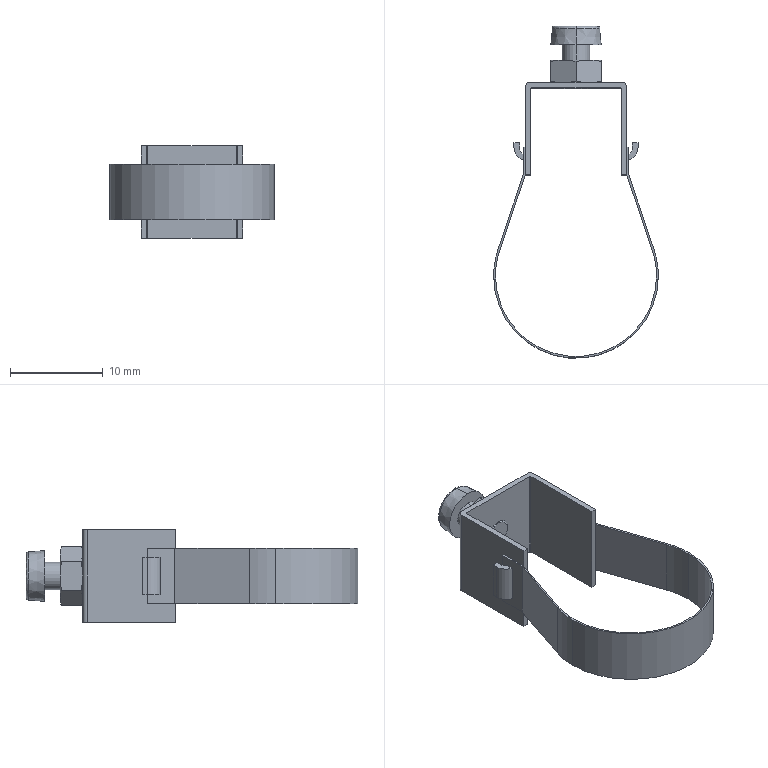Part | STEP file | QA-HI_SBA16-SM_3 | 1 solid | 89 faces | box 17.8 x 35.9 x 10 mm | volume 369.6 mm3 | plane 53 | cone 18 | cylinder 16 | spline 2 | commonest cylinder face diameters 3 x4 17.4 x3 17.8 x3 0.2 x2 1 x2 1.8 x2